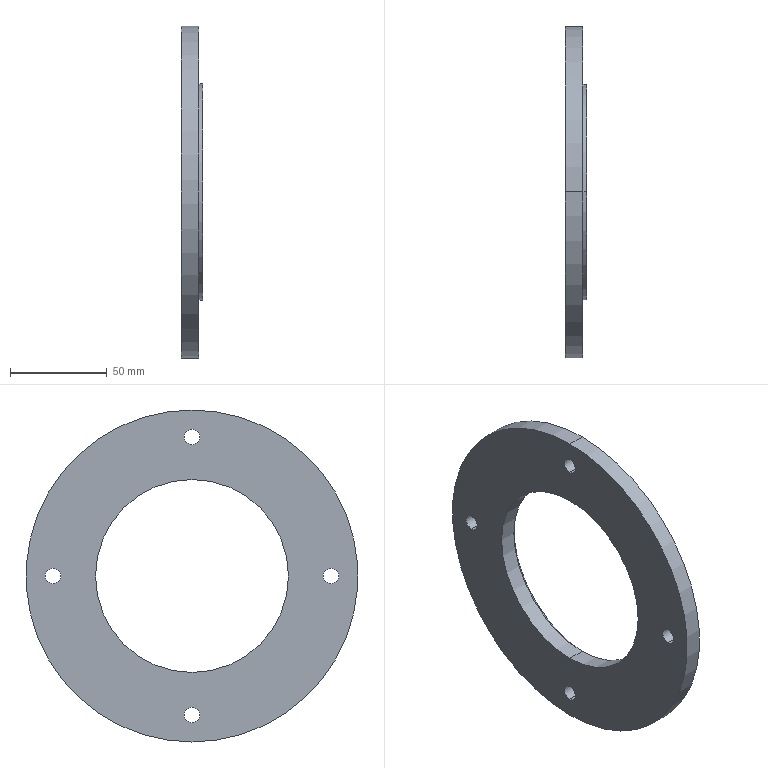Part | NX | features BREP 1 | 1 solid | 19 faces | box 11 x 172 x 172 mm | volume 139981 mm3 | cylinder 14 | plane 3 | cone 2 | commonest cylinder face diameters 8 x8 100 x2 112 x2 172 x2
STEP:
#1=CARTESIAN_POINT('',(9.,0.,-68.));
#2=VERTEX_POINT('',#1);
#3=CARTESIAN_POINT('',(9.,0.,-76.));
#4=VERTEX_POINT('',#3);
#5=CARTESIAN_POINT('',(9.,0.,-72.));
#6=DIRECTION('',(1.,0.,0.));
#7=DIRECTION('',(0.,0.,1.));
#8=AXIS2_PLACEMENT_3D('',#5,#6,#7);
#9=CIRCLE('',#8,4.);
#10=EDGE_CURVE('',#2,#4,#9,.T.);
#11=ORIENTED_EDGE('',*,*,#10,.T.);
#12=CARTESIAN_POINT('',(0.,0.,-76.));
#13=VERTEX_POINT('',#12);
#14=CARTESIAN_POINT('',(11.001,0.,-76.));
#15=DIRECTION('',(-1.,0.,0.));
#16=VECTOR('',#15,1000.);
#17=LINE('',#14,#16);
#18=EDGE_CURVE('',#4,#13,#17,.T.);
#19=ORIENTED_EDGE('',*,*,#18,.T.);
#20=CARTESIAN_POINT('',(0.,0.,-68.));
#21=VERTEX_POINT('',#20);
#22=CARTESIAN_POINT('',(0.,0.,-72.));
#23=DIRECTION('',(-1.,0.,0.));
#24=DIRECTION('',(0.,0.,1.));
#25=AXIS2_PLACEMENT_3D('',#22,#23,#24);
#26=CIRCLE('',#25,4.);
#27=EDGE_CURVE('',#13,#21,#26,.T.);
#28=ORIENTED_EDGE('',*,*,#27,.T.);
#29=CARTESIAN_POINT('',(11.001,0.,-68.));
#30=DIRECTION('',(-1.,0.,0.));
#31=VECTOR('',#30,1000.);
#32=LINE('',#29,#31);
#33=EDGE_CURVE('',#2,#21,#32,.T.);
#34=ORIENTED_EDGE('',*,*,#33,.F.);
#35=EDGE_LOOP('',(#11,#19,#28,#34));
#36=FACE_BOUND('',#35,.T.);
#37=CARTESIAN_POINT('',(11.001,0.,-72.));
#38=DIRECTION('',(-1.,0.,0.));
#39=DIRECTION('',(0.,0.,-1.));
#40=AXIS2_PLACEMENT_3D('',#37,#38,#39);
#41=CYLINDRICAL_SURFACE('',#40,4.);
#42=ADVANCED_FACE('',(#36),#41,.F.);
#43=CARTESIAN_POINT('',(9.,-72.,4.));
#44=VERTEX_POINT('',#43);
#45=CARTESIAN_POINT('',(9.,-72.,-4.));
#46=VERTEX_POINT('',#45);
#47=CARTESIAN_POINT('',(9.,-72.,0.));
#48=DIRECTION('',(1.,0.,0.));
#49=DIRECTION('',(0.,0.,1.));
#50=AXIS2_PLACEMENT_3D('',#47,#48,#49);
#51=CIRCLE('',#50,4.);
#52=EDGE_CURVE('',#44,#46,#51,.T.);
#53=ORIENTED_EDGE('',*,*,#52,.T.);
#54=CARTESIAN_POINT('',(0.,-72.,-4.));
#55=VERTEX_POINT('',#54);
#56=CARTESIAN_POINT('',(11.001,-72.,-4.));
#57=DIRECTION('',(-1.,0.,0.));
#58=VECTOR('',#57,1000.);
#59=LINE('',#56,#58);
#60=EDGE_CURVE('',#46,#55,#59,.T.);
#61=ORIENTED_EDGE('',*,*,#60,.T.);
#62=CARTESIAN_POINT('',(0.,-72.,4.));
#63=VERTEX_POINT('',#62);
#64=CARTESIAN_POINT('',(0.,-72.,0.));
#65=DIRECTION('',(-1.,0.,0.));
#66=DIRECTION('',(0.,0.,1.));
#67=AXIS2_PLACEMENT_3D('',#64,#65,#66);
#68=CIRCLE('',#67,4.);
#69=EDGE_CURVE('',#55,#63,#68,.T.);
#70=ORIENTED_EDGE('',*,*,#69,.T.);
#71=CARTESIAN_POINT('',(11.001,-72.,4.));
#72=DIRECTION('',(-1.,0.,0.));
#73=VECTOR('',#72,1000.);
#74=LINE('',#71,#73);
#75=EDGE_CURVE('',#44,#63,#74,.T.);
#76=ORIENTED_EDGE('',*,*,#75,.F.);
#77=EDGE_LOOP('',(#53,#61,#70,#76));
#78=FACE_BOUND('',#77,.T.);
#79=CARTESIAN_POINT('',(11.001,-72.,0.));
#80=DIRECTION('',(-1.,0.,0.));
#81=DIRECTION('',(0.,0.,-1.));
#82=AXIS2_PLACEMENT_3D('',#79,#80,#81);
#83=CYLINDRICAL_SURFACE('',#82,4.);
#84=ADVANCED_FACE('',(#78),#83,.F.);
#85=CARTESIAN_POINT('',(9.,0.,76.));
#86=VERTEX_POINT('',#85);
#87=CARTESIAN_POINT('',(9.,0.,68.));
#88=VERTEX_POINT('',#87);
#89=CARTESIAN_POINT('',(9.,0.,72.));
#90=DIRECTION('',(1.,0.,0.));
#91=DIRECTION('',(0.,0.,1.));
#92=AXIS2_PLACEMENT_3D('',#89,#90,#91);
#93=CIRCLE('',#92,4.);
#94=EDGE_CURVE('',#86,#88,#93,.T.);
#95=ORIENTED_EDGE('',*,*,#94,.T.);
#96=CARTESIAN_POINT('',(0.,0.,68.));
#97=VERTEX_POINT('',#96);
#98=CARTESIAN_POINT('',(11.001,0.,68.));
#99=DIRECTION('',(-1.,0.,0.));
#100=VECTOR('',#99,1000.);
#101=LINE('',#98,#100);
#102=EDGE_CURVE('',#88,#97,#101,.T.);
#103=ORIENTED_EDGE('',*,*,#102,.T.);
#104=CARTESIAN_POINT('',(0.,0.,76.));
#105=VERTEX_POINT('',#104);
#106=CARTESIAN_POINT('',(0.,0.,72.));
#107=DIRECTION('',(-1.,0.,0.));
#108=DIRECTION('',(0.,0.,1.));
#109=AXIS2_PLACEMENT_3D('',#106,#107,#108);
#110=CIRCLE('',#109,4.);
#111=EDGE_CURVE('',#97,#105,#110,.T.);
#112=ORIENTED_EDGE('',*,*,#111,.T.);
#113=CARTESIAN_POINT('',(11.001,0.,76.));
#114=DIRECTION('',(-1.,0.,0.));
#115=VECTOR('',#114,1000.);
#116=LINE('',#113,#115);
#117=EDGE_CURVE('',#86,#105,#116,.T.);
#118=ORIENTED_EDGE('',*,*,#117,.F.);
#119=EDGE_LOOP('',(#95,#103,#112,#118));
#120=FACE_BOUND('',#119,.T.);
#121=CARTESIAN_POINT('',(11.001,0.,72.));
#122=DIRECTION('',(-1.,0.,0.));
#123=DIRECTION('',(0.,0.,-1.));
#124=AXIS2_PLACEMENT_3D('',#121,#122,#123);
#125=CYLINDRICAL_SURFACE('',#124,4.);
#126=ADVANCED_FACE('',(#120),#125,.F.);
#127=CARTESIAN_POINT('',(9.,72.,4.));
#128=VERTEX_POINT('',#127);
#129=CARTESIAN_POINT('',(9.,72.,-4.));
#130=VERTEX_POINT('',#129);
#131=CARTESIAN_POINT('',(9.,72.,0.));
#132=DIRECTION('',(1.,0.,0.));
#133=DIRECTION('',(0.,0.,1.));
#134=AXIS2_PLACEMENT_3D('',#131,#132,#133);
#135=CIRCLE('',#134,4.);
#136=EDGE_CURVE('',#128,#130,#135,.T.);
#137=ORIENTED_EDGE('',*,*,#136,.T.);
#138=CARTESIAN_POINT('',(0.,72.,-4.));
#139=VERTEX_POINT('',#138);
#140=CARTESIAN_POINT('',(11.001,72.,-4.));
#141=DIRECTION('',(-1.,0.,0.));
#142=VECTOR('',#141,1000.);
#143=LINE('',#140,#142);
#144=EDGE_CURVE('',#130,#139,#143,.T.);
#145=ORIENTED_EDGE('',*,*,#144,.T.);
#146=CARTESIAN_POINT('',(0.,72.,4.));
#147=VERTEX_POINT('',#146);
#148=CARTESIAN_POINT('',(0.,72.,0.));
#149=DIRECTION('',(-1.,0.,0.));
#150=DIRECTION('',(0.,0.,1.));
#151=AXIS2_PLACEMENT_3D('',#148,#149,#150);
#152=CIRCLE('',#151,4.);
#153=EDGE_CURVE('',#139,#147,#152,.T.);
#154=ORIENTED_EDGE('',*,*,#153,.T.);
#155=CARTESIAN_POINT('',(11.001,72.,4.));
#156=DIRECTION('',(-1.,0.,0.));
#157=VECTOR('',#156,1000.);
#158=LINE('',#155,#157);
#159=EDGE_CURVE('',#128,#147,#158,.T.);
#160=ORIENTED_EDGE('',*,*,#159,.F.);
#161=EDGE_LOOP('',(#137,#145,#154,#160));
#162=FACE_BOUND('',#161,.T.);
#163=CARTESIAN_POINT('',(11.001,72.,0.));
#164=DIRECTION('',(-1.,0.,0.));
#165=DIRECTION('',(0.,0.,-1.));
#166=AXIS2_PLACEMENT_3D('',#163,#164,#165);
#167=CYLINDRICAL_SURFACE('',#166,4.);
#168=ADVANCED_FACE('',(#162),#167,.F.);
#169=CARTESIAN_POINT('',(9.,0.,-50.));
#170=VERTEX_POINT('',#169);
#171=CARTESIAN_POINT('',(9.,0.,50.));
#172=VERTEX_POINT('',#171);
#173=CARTESIAN_POINT('',(9.,0.,0.));
#174=DIRECTION('',(-1.,0.,0.));
#175=DIRECTION('',(0.,0.,1.));
#176=AXIS2_PLACEMENT_3D('',#173,#174,#175);
#177=CIRCLE('',#176,50.);
#178=EDGE_CURVE('',#170,#172,#177,.T.);
#179=ORIENTED_EDGE('',*,*,#178,.T.);
#180=CARTESIAN_POINT('',(11.,0.,52.));
#181=VERTEX_POINT('',#180);
#182=CARTESIAN_POINT('',(9.,0.,50.));
#183=DIRECTION('',(0.7071,0.,0.7071));
#184=VECTOR('',#183,1000.);
#185=LINE('',#182,#184);
#186=EDGE_CURVE('',#181,#172,#185,.F.);
#187=ORIENTED_EDGE('',*,*,#186,.F.);
#188=CARTESIAN_POINT('',(11.,0.,-52.));
#189=VERTEX_POINT('',#188);
#190=CARTESIAN_POINT('',(11.,0.,0.));
#191=DIRECTION('',(-1.,0.,0.));
#192=DIRECTION('',(0.,0.,1.));
#193=AXIS2_PLACEMENT_3D('',#190,#191,#192);
#194=CIRCLE('',#193,52.);
#195=EDGE_CURVE('',#189,#181,#194,.T.);
#196=ORIENTED_EDGE('',*,*,#195,.F.);
#197=CARTESIAN_POINT('',(9.,0.,-50.));
#198=DIRECTION('',(0.7071,0.,-0.7071));
#199=VECTOR('',#198,1000.);
#200=LINE('',#197,#199);
#201=EDGE_CURVE('',#189,#170,#200,.F.);
#202=ORIENTED_EDGE('',*,*,#201,.T.);
#203=EDGE_LOOP('',(#179,#187,#196,#202));
#204=FACE_BOUND('',#203,.T.);
#205=CARTESIAN_POINT('',(9.,0.,0.));
#206=DIRECTION('',(1.,0.,0.));
#207=DIRECTION('',(0.,0.,1.));
#208=AXIS2_PLACEMENT_3D('',#205,#206,#207);
#209=CONICAL_SURFACE('',#208,50.,0.7854);
#210=ADVANCED_FACE('',(#204),#209,.F.);
#211=CARTESIAN_POINT('',(11.,0.,56.));
#212=VERTEX_POINT('',#211);
#213=CARTESIAN_POINT('',(11.,0.,-56.));
#214=VERTEX_POINT('',#213);
#215=CARTESIAN_POINT('',(11.,0.,0.));
#216=DIRECTION('',(-1.,0.,0.));
#217=DIRECTION('',(0.,0.,1.));
#218=AXIS2_PLACEMENT_3D('',#215,#216,#217);
#219=CIRCLE('',#218,56.);
#220=EDGE_CURVE('',#212,#214,#219,.T.);
#221=ORIENTED_EDGE('',*,*,#220,.T.);
#222=CARTESIAN_POINT('',(9.,0.,-56.));
#223=VERTEX_POINT('',#222);
#224=CARTESIAN_POINT('',(0.,0.,-56.));
#225=DIRECTION('',(-1.,0.,0.));
#226=VECTOR('',#225,1000.);
#227=LINE('',#224,#226);
#228=EDGE_CURVE('',#214,#223,#227,.T.);
#229=ORIENTED_EDGE('',*,*,#228,.T.);
#230=CARTESIAN_POINT('',(9.,0.,56.));
#231=VERTEX_POINT('',#230);
#232=CARTESIAN_POINT('',(9.,0.,0.));
#233=DIRECTION('',(-1.,0.,0.));
#234=DIRECTION('',(0.,0.,1.));
#235=AXIS2_PLACEMENT_3D('',#232,#233,#234);
#236=CIRCLE('',#235,56.);
#237=EDGE_CURVE('',#231,#223,#236,.T.);
#238=ORIENTED_EDGE('',*,*,#237,.F.);
#239=CARTESIAN_POINT('',(0.,0.,56.));
#240=DIRECTION('',(-1.,0.,0.));
#241=VECTOR('',#240,1000.);
#242=LINE('',#239,#241);
#243=EDGE_CURVE('',#212,#231,#242,.T.);
#244=ORIENTED_EDGE('',*,*,#243,.F.);
#245=EDGE_LOOP('',(#221,#229,#238,#244));
#246=FACE_BOUND('',#245,.T.);
#247=CARTESIAN_POINT('',(0.,0.,0.));
#248=DIRECTION('',(-1.,0.,0.));
#249=DIRECTION('',(0.,0.,-1.));
#250=AXIS2_PLACEMENT_3D('',#247,#248,#249);
#251=CYLINDRICAL_SURFACE('',#250,56.);
#252=ADVANCED_FACE('',(#246),#251,.T.);
#253=CARTESIAN_POINT('',(9.,0.,86.));
#254=VERTEX_POINT('',#253);
#255=CARTESIAN_POINT('',(9.,0.,-86.));
#256=VERTEX_POINT('',#255);
#257=CARTESIAN_POINT('',(9.,0.,0.));
#258=DIRECTION('',(-1.,0.,0.));
#259=DIRECTION('',(0.,0.,1.));
#260=AXIS2_PLACEMENT_3D('',#257,#258,#259);
#261=CIRCLE('',#260,86.);
#262=EDGE_CURVE('',#254,#256,#261,.T.);
#263=ORIENTED_EDGE('',*,*,#262,.T.);
#264=CARTESIAN_POINT('',(0.,0.,-86.));
#265=VERTEX_POINT('',#264);
#266=CARTESIAN_POINT('',(0.,0.,-86.));
#267=DIRECTION('',(-1.,0.,0.));
#268=VECTOR('',#267,1000.);
#269=LINE('',#266,#268);
#270=EDGE_CURVE('',#256,#265,#269,.T.);
#271=ORIENTED_EDGE('',*,*,#270,.T.);
#272=CARTESIAN_POINT('',(0.,0.,86.));
#273=VERTEX_POINT('',#272);
#274=CARTESIAN_POINT('',(0.,0.,0.));
#275=DIRECTION('',(-1.,0.,0.));
#276=DIRECTION('',(0.,0.,1.));
#277=AXIS2_PLACEMENT_3D('',#274,#275,#276);
#278=CIRCLE('',#277,86.);
#279=EDGE_CURVE('',#273,#265,#278,.T.);
#280=ORIENTED_EDGE('',*,*,#279,.F.);
#281=CARTESIAN_POINT('',(0.,0.,86.));
#282=DIRECTION('',(-1.,0.,0.));
#283=VECTOR('',#282,1000.);
#284=LINE('',#281,#283);
#285=EDGE_CURVE('',#254,#273,#284,.T.);
#286=ORIENTED_EDGE('',*,*,#285,.F.);
#287=EDGE_LOOP('',(#263,#271,#280,#286));
#288=FACE_BOUND('',#287,.T.);
#289=CARTESIAN_POINT('',(0.,0.,0.));
#290=DIRECTION('',(-1.,0.,0.));
#291=DIRECTION('',(0.,0.,-1.));
#292=AXIS2_PLACEMENT_3D('',#289,#290,#291);
#293=CYLINDRICAL_SURFACE('',#292,86.);
#294=ADVANCED_FACE('',(#288),#293,.T.);
#295=ORIENTED_EDGE('',*,*,#178,.F.);
#296=CARTESIAN_POINT('',(0.,0.,-50.));
#297=VERTEX_POINT('',#296);
#298=CARTESIAN_POINT('',(0.,0.,-50.));
#299=DIRECTION('',(-1.,0.,0.));
#300=VECTOR('',#299,1000.);
#301=LINE('',#298,#300);
#302=EDGE_CURVE('',#170,#297,#301,.T.);
#303=ORIENTED_EDGE('',*,*,#302,.T.);
#304=CARTESIAN_POINT('',(0.,0.,50.));
#305=VERTEX_POINT('',#304);
#306=CARTESIAN_POINT('',(0.,0.,0.));
#307=DIRECTION('',(-1.,0.,0.));
#308=DIRECTION('',(0.,0.,1.));
#309=AXIS2_PLACEMENT_3D('',#306,#307,#308);
#310=CIRCLE('',#309,50.);
#311=EDGE_CURVE('',#297,#305,#310,.T.);
#312=ORIENTED_EDGE('',*,*,#311,.T.);
#313=CARTESIAN_POINT('',(0.,0.,50.));
#314=DIRECTION('',(-1.,0.,0.));
#315=VECTOR('',#314,1000.);
#316=LINE('',#313,#315);
#317=EDGE_CURVE('',#172,#305,#316,.T.);
#318=ORIENTED_EDGE('',*,*,#317,.F.);
#319=EDGE_LOOP('',(#295,#303,#312,#318));
#320=FACE_BOUND('',#319,.T.);
#321=CARTESIAN_POINT('',(0.,0.,0.));
#322=DIRECTION('',(-1.,0.,0.));
#323=DIRECTION('',(0.,0.,-1.));
#324=AXIS2_PLACEMENT_3D('',#321,#322,#323);
#325=CYLINDRICAL_SURFACE('',#324,50.);
#326=ADVANCED_FACE('',(#320),#325,.F.);
#327=ORIENTED_EDGE('',*,*,#302,.F.);
#328=CARTESIAN_POINT('',(9.,0.,0.));
#329=DIRECTION('',(-1.,0.,0.));
#330=DIRECTION('',(0.,0.,1.));
#331=AXIS2_PLACEMENT_3D('',#328,#329,#330);
#332=CIRCLE('',#331,50.);
#333=EDGE_CURVE('',#172,#170,#332,.T.);
#334=ORIENTED_EDGE('',*,*,#333,.F.);
#335=ORIENTED_EDGE('',*,*,#317,.T.);
#336=CARTESIAN_POINT('',(0.,0.,0.));
#337=DIRECTION('',(-1.,0.,0.));
#338=DIRECTION('',(0.,0.,1.));
#339=AXIS2_PLACEMENT_3D('',#336,#337,#338);
#340=CIRCLE('',#339,50.);
#341=EDGE_CURVE('',#305,#297,#340,.T.);
#342=ORIENTED_EDGE('',*,*,#341,.T.);
#343=EDGE_LOOP('',(#327,#334,#335,#342));
#344=FACE_BOUND('',#343,.T.);
#345=CARTESIAN_POINT('',(0.,0.,0.));
#346=DIRECTION('',(-1.,0.,0.));
#347=DIRECTION('',(0.,0.,-1.));
#348=AXIS2_PLACEMENT_3D('',#345,#346,#347);
#349=CYLINDRICAL_SURFACE('',#348,50.);
#350=ADVANCED_FACE('',(#344),#349,.F.);
#351=ORIENTED_EDGE('',*,*,#279,.T.);
#352=CARTESIAN_POINT('',(0.,0.,0.));
#353=DIRECTION('',(-1.,0.,0.));
#354=DIRECTION('',(0.,0.,1.));
#355=AXIS2_PLACEMENT_3D('',#352,#353,#354);
#356=CIRCLE('',#355,86.);
#357=EDGE_CURVE('',#265,#273,#356,.T.);
#358=ORIENTED_EDGE('',*,*,#357,.T.);
#359=EDGE_LOOP('',(#351,#358));
#360=FACE_BOUND('',#359,.T.);
#361=CARTESIAN_POINT('',(0.,0.,-72.));
#362=DIRECTION('',(-1.,0.,0.));
#363=DIRECTION('',(0.,0.,1.));
#364=AXIS2_PLACEMENT_3D('',#361,#362,#363);
#365=CIRCLE('',#364,4.);
#366=EDGE_CURVE('',#21,#13,#365,.T.);
#367=ORIENTED_EDGE('',*,*,#366,.F.);
#368=ORIENTED_EDGE('',*,*,#27,.F.);
#369=EDGE_LOOP('',(#367,#368));
#370=FACE_BOUND('',#369,.T.);
#371=CARTESIAN_POINT('',(0.,-72.,0.));
#372=DIRECTION('',(-1.,0.,0.));
#373=DIRECTION('',(0.,0.,1.));
#374=AXIS2_PLACEMENT_3D('',#371,#372,#373);
#375=CIRCLE('',#374,4.);
#376=EDGE_CURVE('',#63,#55,#375,.T.);
#377=ORIENTED_EDGE('',*,*,#376,.F.);
#378=ORIENTED_EDGE('',*,*,#69,.F.);
#379=EDGE_LOOP('',(#377,#378));
#380=FACE_BOUND('',#379,.T.);
#381=CARTESIAN_POINT('',(0.,0.,72.));
#382=DIRECTION('',(-1.,0.,0.));
#383=DIRECTION('',(0.,0.,1.));
#384=AXIS2_PLACEMENT_3D('',#381,#382,#383);
#385=CIRCLE('',#384,4.);
#386=EDGE_CURVE('',#105,#97,#385,.T.);
#387=ORIENTED_EDGE('',*,*,#386,.F.);
#388=ORIENTED_EDGE('',*,*,#111,.F.);
#389=EDGE_LOOP('',(#387,#388));
#390=FACE_BOUND('',#389,.T.);
#391=CARTESIAN_POINT('',(0.,72.,0.));
#392=DIRECTION('',(-1.,0.,0.));
#393=DIRECTION('',(0.,0.,1.));
#394=AXIS2_PLACEMENT_3D('',#391,#392,#393);
#395=CIRCLE('',#394,4.);
#396=EDGE_CURVE('',#147,#139,#395,.T.);
#397=ORIENTED_EDGE('',*,*,#396,.F.);
#398=ORIENTED_EDGE('',*,*,#153,.F.);
#399=EDGE_LOOP('',(#397,#398));
#400=FACE_BOUND('',#399,.T.);
#401=ORIENTED_EDGE('',*,*,#341,.F.);
#402=ORIENTED_EDGE('',*,*,#311,.F.);
#403=EDGE_LOOP('',(#401,#402));
#404=FACE_BOUND('',#403,.T.);
#405=CARTESIAN_POINT('',(0.,50.,0.));
#406=DIRECTION('',(1.,0.,0.));
#407=DIRECTION('',(0.,1.,0.));
#408=AXIS2_PLACEMENT_3D('',#405,#406,#407);
#409=PLANE('',#408);
#410=ADVANCED_FACE('',(#360,#370,#380,#390,#400,#404),#409,.F.);
#411=ORIENTED_EDGE('',*,*,#270,.F.);
#412=CARTESIAN_POINT('',(9.,0.,0.));
#413=DIRECTION('',(-1.,0.,0.));
#414=DIRECTION('',(0.,0.,1.));
#415=AXIS2_PLACEMENT_3D('',#412,#413,#414);
#416=CIRCLE('',#415,86.);
#417=EDGE_CURVE('',#256,#254,#416,.T.);
#418=ORIENTED_EDGE('',*,*,#417,.T.);
#419=ORIENTED_EDGE('',*,*,#285,.T.);
#420=ORIENTED_EDGE('',*,*,#357,.F.);
#421=EDGE_LOOP('',(#411,#418,#419,#420));
#422=FACE_BOUND('',#421,.T.);
#423=CARTESIAN_POINT('',(0.,0.,0.));
#424=DIRECTION('',(-1.,0.,0.));
#425=DIRECTION('',(0.,0.,-1.));
#426=AXIS2_PLACEMENT_3D('',#423,#424,#425);
#427=CYLINDRICAL_SURFACE('',#426,86.);
#428=ADVANCED_FACE('',(#422),#427,.T.);
#429=ORIENTED_EDGE('',*,*,#262,.F.);
#430=ORIENTED_EDGE('',*,*,#417,.F.);
#431=EDGE_LOOP('',(#429,#430));
#432=FACE_BOUND('',#431,.T.);
#433=ORIENTED_EDGE('',*,*,#10,.F.);
#434=CARTESIAN_POINT('',(9.,0.,-72.));
#435=DIRECTION('',(1.,0.,0.));
#436=DIRECTION('',(0.,0.,1.));
#437=AXIS2_PLACEMENT_3D('',#434,#435,#436);
#438=CIRCLE('',#437,4.);
#439=EDGE_CURVE('',#4,#2,#438,.T.);
#440=ORIENTED_EDGE('',*,*,#439,.F.);
#441=EDGE_LOOP('',(#433,#440));
#442=FACE_BOUND('',#441,.T.);
#443=ORIENTED_EDGE('',*,*,#52,.F.);
#444=CARTESIAN_POINT('',(9.,-72.,0.));
#445=DIRECTION('',(1.,0.,0.));
#446=DIRECTION('',(0.,0.,1.));
#447=AXIS2_PLACEMENT_3D('',#444,#445,#446);
#448=CIRCLE('',#447,4.);
#449=EDGE_CURVE('',#46,#44,#448,.T.);
#450=ORIENTED_EDGE('',*,*,#449,.F.);
#451=EDGE_LOOP('',(#443,#450));
#452=FACE_BOUND('',#451,.T.);
#453=ORIENTED_EDGE('',*,*,#94,.F.);
#454=CARTESIAN_POINT('',(9.,0.,72.));
#455=DIRECTION('',(1.,0.,0.));
#456=DIRECTION('',(0.,0.,1.));
#457=AXIS2_PLACEMENT_3D('',#454,#455,#456);
#458=CIRCLE('',#457,4.);
#459=EDGE_CURVE('',#88,#86,#458,.T.);
#460=ORIENTED_EDGE('',*,*,#459,.F.);
#461=EDGE_LOOP('',(#453,#460));
#462=FACE_BOUND('',#461,.T.);
#463=ORIENTED_EDGE('',*,*,#136,.F.);
#464=CARTESIAN_POINT('',(9.,72.,0.));
#465=DIRECTION('',(1.,0.,0.));
#466=DIRECTION('',(0.,0.,1.));
#467=AXIS2_PLACEMENT_3D('',#464,#465,#466);
#468=CIRCLE('',#467,4.);
#469=EDGE_CURVE('',#130,#128,#468,.T.);
#470=ORIENTED_EDGE('',*,*,#469,.F.);
#471=EDGE_LOOP('',(#463,#470));
#472=FACE_BOUND('',#471,.T.);
#473=ORIENTED_EDGE('',*,*,#237,.T.);
#474=CARTESIAN_POINT('',(9.,0.,0.));
#475=DIRECTION('',(-1.,0.,0.));
#476=DIRECTION('',(0.,0.,1.));
#477=AXIS2_PLACEMENT_3D('',#474,#475,#476);
#478=CIRCLE('',#477,56.);
#479=EDGE_CURVE('',#223,#231,#478,.T.);
#480=ORIENTED_EDGE('',*,*,#479,.T.);
#481=EDGE_LOOP('',(#473,#480));
#482=FACE_BOUND('',#481,.T.);
#483=CARTESIAN_POINT('',(9.,86.,0.));
#484=DIRECTION('',(-1.,0.,0.));
#485=DIRECTION('',(0.,0.,-1.));
#486=AXIS2_PLACEMENT_3D('',#483,#484,#485);
#487=PLANE('',#486);
#488=ADVANCED_FACE('',(#432,#442,#452,#462,#472,#482),#487,.F.);
#489=ORIENTED_EDGE('',*,*,#228,.F.);
#490=CARTESIAN_POINT('',(11.,0.,0.));
#491=DIRECTION('',(-1.,0.,0.));
#492=DIRECTION('',(0.,0.,1.));
#493=AXIS2_PLACEMENT_3D('',#490,#491,#492);
#494=CIRCLE('',#493,56.);
#495=EDGE_CURVE('',#214,#212,#494,.T.);
#496=ORIENTED_EDGE('',*,*,#495,.T.);
#497=ORIENTED_EDGE('',*,*,#243,.T.);
#498=ORIENTED_EDGE('',*,*,#479,.F.);
#499=EDGE_LOOP('',(#489,#496,#497,#498));
#500=FACE_BOUND('',#499,.T.);
#501=CARTESIAN_POINT('',(0.,0.,0.));
#502=DIRECTION('',(-1.,0.,0.));
#503=DIRECTION('',(0.,0.,-1.));
#504=AXIS2_PLACEMENT_3D('',#501,#502,#503);
#505=CYLINDRICAL_SURFACE('',#504,56.);
#506=ADVANCED_FACE('',(#500),#505,.T.);
#507=ORIENTED_EDGE('',*,*,#220,.F.);
#508=ORIENTED_EDGE('',*,*,#495,.F.);
#509=EDGE_LOOP('',(#507,#508));
#510=FACE_BOUND('',#509,.T.);
#511=ORIENTED_EDGE('',*,*,#195,.T.);
#512=CARTESIAN_POINT('',(11.,0.,0.));
#513=DIRECTION('',(-1.,0.,0.));
#514=DIRECTION('',(0.,0.,1.));
#515=AXIS2_PLACEMENT_3D('',#512,#513,#514);
#516=CIRCLE('',#515,52.);
#517=EDGE_CURVE('',#181,#189,#516,.T.);
#518=ORIENTED_EDGE('',*,*,#517,.T.);
#519=EDGE_LOOP('',(#511,#518));
#520=FACE_BOUND('',#519,.T.);
#521=CARTESIAN_POINT('',(11.,56.,0.));
#522=DIRECTION('',(-1.,0.,0.));
#523=DIRECTION('',(0.,0.,-1.));
#524=AXIS2_PLACEMENT_3D('',#521,#522,#523);
#525=PLANE('',#524);
#526=ADVANCED_FACE('',(#510,#520),#525,.F.);
#527=ORIENTED_EDGE('',*,*,#186,.T.);
#528=ORIENTED_EDGE('',*,*,#333,.T.);
#529=ORIENTED_EDGE('',*,*,#201,.F.);
#530=ORIENTED_EDGE('',*,*,#517,.F.);
#531=EDGE_LOOP('',(#527,#528,#529,#530));
#532=FACE_BOUND('',#531,.T.);
#533=CARTESIAN_POINT('',(9.,0.,0.));
#534=DIRECTION('',(1.,0.,0.));
#535=DIRECTION('',(0.,0.,1.));
#536=AXIS2_PLACEMENT_3D('',#533,#534,#535);
#537=CONICAL_SURFACE('',#536,50.,0.7854);
#538=ADVANCED_FACE('',(#532),#537,.F.);
#539=ORIENTED_EDGE('',*,*,#144,.F.);
#540=ORIENTED_EDGE('',*,*,#469,.T.);
#541=ORIENTED_EDGE('',*,*,#159,.T.);
#542=ORIENTED_EDGE('',*,*,#396,.T.);
#543=EDGE_LOOP('',(#539,#540,#541,#542));
#544=FACE_BOUND('',#543,.T.);
#545=CARTESIAN_POINT('',(11.001,72.,0.));
#546=DIRECTION('',(-1.,0.,0.));
#547=DIRECTION('',(0.,0.,-1.));
#548=AXIS2_PLACEMENT_3D('',#545,#546,#547);
#549=CYLINDRICAL_SURFACE('',#548,4.);
#550=ADVANCED_FACE('',(#544),#549,.F.);
#551=ORIENTED_EDGE('',*,*,#102,.F.);
#552=ORIENTED_EDGE('',*,*,#459,.T.);
#553=ORIENTED_EDGE('',*,*,#117,.T.);
#554=ORIENTED_EDGE('',*,*,#386,.T.);
#555=EDGE_LOOP('',(#551,#552,#553,#554));
#556=FACE_BOUND('',#555,.T.);
#557=CARTESIAN_POINT('',(11.001,0.,72.));
#558=DIRECTION('',(-1.,0.,0.));
#559=DIRECTION('',(0.,0.,-1.));
#560=AXIS2_PLACEMENT_3D('',#557,#558,#559);
#561=CYLINDRICAL_SURFACE('',#560,4.);
#562=ADVANCED_FACE('',(#556),#561,.F.);
#563=ORIENTED_EDGE('',*,*,#60,.F.);
#564=ORIENTED_EDGE('',*,*,#449,.T.);
#565=ORIENTED_EDGE('',*,*,#75,.T.);
#566=ORIENTED_EDGE('',*,*,#376,.T.);
#567=EDGE_LOOP('',(#563,#564,#565,#566));
#568=FACE_BOUND('',#567,.T.);
#569=CARTESIAN_POINT('',(11.001,-72.,0.));
#570=DIRECTION('',(-1.,0.,0.));
#571=DIRECTION('',(0.,0.,-1.));
#572=AXIS2_PLACEMENT_3D('',#569,#570,#571);
#573=CYLINDRICAL_SURFACE('',#572,4.);
#574=ADVANCED_FACE('',(#568),#573,.F.);
#575=ORIENTED_EDGE('',*,*,#18,.F.);
#576=ORIENTED_EDGE('',*,*,#439,.T.);
#577=ORIENTED_EDGE('',*,*,#33,.T.);
#578=ORIENTED_EDGE('',*,*,#366,.T.);
#579=EDGE_LOOP('',(#575,#576,#577,#578));
#580=FACE_BOUND('',#579,.T.);
#581=CARTESIAN_POINT('',(11.001,0.,-72.));
#582=DIRECTION('',(-1.,0.,0.));
#583=DIRECTION('',(0.,0.,-1.));
#584=AXIS2_PLACEMENT_3D('',#581,#582,#583);
#585=CYLINDRICAL_SURFACE('',#584,4.);
#586=ADVANCED_FACE('',(#580),#585,.F.);
#587=CLOSED_SHELL('',(#42,#84,#126,#168,#210,#252,#294,#326,#350,#410,#428,#488,#506,#526,#538,#550,#562,#574,#586));
#588=MANIFOLD_SOLID_BREP('',#587);
#589=(LENGTH_UNIT()NAMED_UNIT(*)SI_UNIT(.MILLI.,.METRE.));
#590=UNCERTAINTY_MEASURE_WITH_UNIT(LENGTH_MEASURE(0.00001),#589,'','');
#591=(NAMED_UNIT(*)PLANE_ANGLE_UNIT()SI_UNIT($,.RADIAN.));
#592=(NAMED_UNIT(*)SI_UNIT($,.STERADIAN.)SOLID_ANGLE_UNIT());
#593=(GEOMETRIC_REPRESENTATION_CONTEXT(3)GLOBAL_UNCERTAINTY_ASSIGNED_CONTEXT((#590))GLOBAL_UNIT_ASSIGNED_CONTEXT((#589,#591,#592))REPRESENTATION_CONTEXT('',''));
#594=ADVANCED_BREP_SHAPE_REPRESENTATION('',(#588),#593);